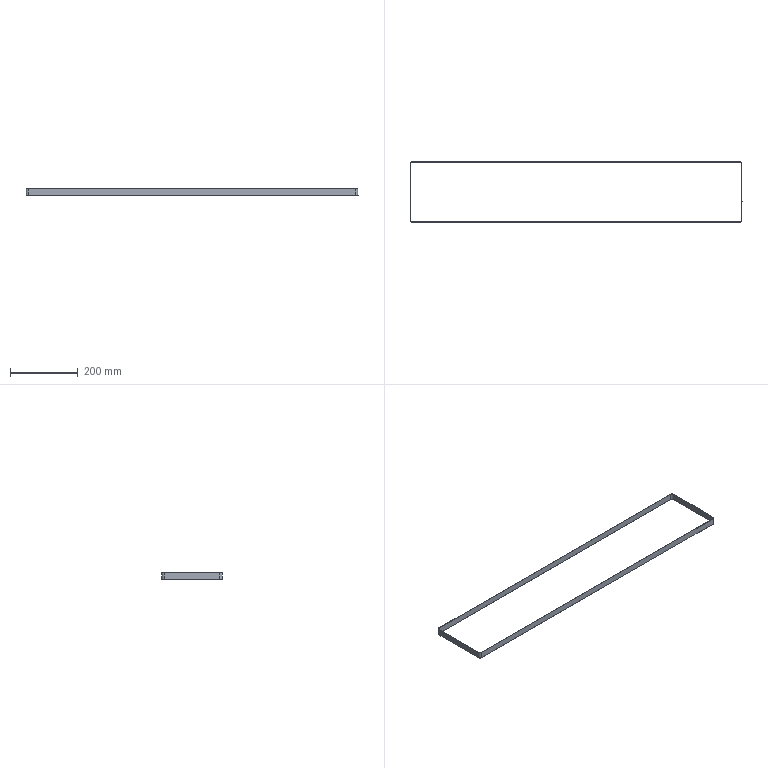Part | NX | features BREP 1 | 1 solid | 26 faces | box 980.9 x 177.8 x 19 mm | volume 35873 mm3 | plane 16 | cylinder 10 | commonest cylinder face diameters 11 x4 12.6 x4 1.64 x2
STEP:
#1=CARTESIAN_POINT('',(483.7,-88.1,0.));
#2=VERTEX_POINT('',#1);
#3=CARTESIAN_POINT('',(483.7,-88.1,-19.));
#4=VERTEX_POINT('',#3);
#5=CARTESIAN_POINT('',(483.7,-88.1,-19.));
#6=DIRECTION('',(0.,0.,-1.));
#7=VECTOR('',#6,1000.);
#8=LINE('',#5,#7);
#9=EDGE_CURVE('',#2,#4,#8,.T.);
#10=ORIENTED_EDGE('',*,*,#9,.T.);
#11=CARTESIAN_POINT('',(-483.7,-88.1,-19.));
#12=VERTEX_POINT('',#11);
#13=CARTESIAN_POINT('',(-483.7,-88.1,-19.));
#14=DIRECTION('',(-1.,0.,0.));
#15=VECTOR('',#14,1000.);
#16=LINE('',#13,#15);
#17=EDGE_CURVE('',#4,#12,#16,.T.);
#18=ORIENTED_EDGE('',*,*,#17,.T.);
#19=CARTESIAN_POINT('',(-483.7,-88.1,0.));
#20=VERTEX_POINT('',#19);
#21=CARTESIAN_POINT('',(-483.7,-88.1,-19.));
#22=DIRECTION('',(0.,0.,1.));
#23=VECTOR('',#22,1000.);
#24=LINE('',#21,#23);
#25=EDGE_CURVE('',#12,#20,#24,.T.);
#26=ORIENTED_EDGE('',*,*,#25,.T.);
#27=CARTESIAN_POINT('',(-483.7,-88.1,0.));
#28=DIRECTION('',(1.,0.,0.));
#29=VECTOR('',#28,1000.);
#30=LINE('',#27,#29);
#31=EDGE_CURVE('',#20,#2,#30,.T.);
#32=ORIENTED_EDGE('',*,*,#31,.T.);
#33=EDGE_LOOP('',(#10,#18,#26,#32));
#34=FACE_BOUND('',#33,.T.);
#35=CARTESIAN_POINT('',(-483.7,-88.1,-19.));
#36=DIRECTION('',(0.,1.,0.));
#37=DIRECTION('',(0.,0.,-1.));
#38=AXIS2_PLACEMENT_3D('',#35,#36,#37);
#39=PLANE('',#38);
#40=ADVANCED_FACE('',(#34),#39,.T.);
#41=CARTESIAN_POINT('',(490.001,-28.898,-19.));
#42=VERTEX_POINT('',#41);
#43=CARTESIAN_POINT('',(490.,-82.6,-19.));
#44=VERTEX_POINT('',#43);
#45=CARTESIAN_POINT('',(490.,-82.6,-19.));
#46=DIRECTION('',(0.,-1.,0.));
#47=VECTOR('',#46,1000.);
#48=LINE('',#45,#47);
#49=EDGE_CURVE('',#42,#44,#48,.T.);
#50=ORIENTED_EDGE('',*,*,#49,.T.);
#51=CARTESIAN_POINT('',(483.7,-88.9,-19.));
#52=VERTEX_POINT('',#51);
#53=CARTESIAN_POINT('',(483.7,-82.6,-19.));
#54=DIRECTION('',(0.,0.,-1.));
#55=DIRECTION('',(1.,0.,0.));
#56=AXIS2_PLACEMENT_3D('',#53,#54,#55);
#57=CIRCLE('',#56,6.3);
#58=EDGE_CURVE('',#44,#52,#57,.T.);
#59=ORIENTED_EDGE('',*,*,#58,.T.);
#60=CARTESIAN_POINT('',(-483.7,-88.9,-19.));
#61=VERTEX_POINT('',#60);
#62=CARTESIAN_POINT('',(489.2,-88.9,-19.));
#63=DIRECTION('',(-1.,0.,0.));
#64=VECTOR('',#63,1000.);
#65=LINE('',#62,#64);
#66=EDGE_CURVE('',#52,#61,#65,.T.);
#67=ORIENTED_EDGE('',*,*,#66,.T.);
#68=CARTESIAN_POINT('',(-490.,-82.6,-19.));
#69=VERTEX_POINT('',#68);
#70=CARTESIAN_POINT('',(-483.7,-82.6,-19.));
#71=DIRECTION('',(0.,0.,-1.));
#72=DIRECTION('',(1.,0.,0.));
#73=AXIS2_PLACEMENT_3D('',#70,#71,#72);
#74=CIRCLE('',#73,6.3);
#75=EDGE_CURVE('',#61,#69,#74,.T.);
#76=ORIENTED_EDGE('',*,*,#75,.T.);
#77=CARTESIAN_POINT('',(-490.,82.6,-19.));
#78=VERTEX_POINT('',#77);
#79=CARTESIAN_POINT('',(-490.,-82.6,-19.));
#80=DIRECTION('',(0.,1.,0.));
#81=VECTOR('',#80,1000.);
#82=LINE('',#79,#81);
#83=EDGE_CURVE('',#69,#78,#82,.T.);
#84=ORIENTED_EDGE('',*,*,#83,.T.);
#85=CARTESIAN_POINT('',(-483.7,88.9,-19.));
#86=VERTEX_POINT('',#85);
#87=CARTESIAN_POINT('',(-483.7,82.6,-19.));
#88=DIRECTION('',(0.,0.,-1.));
#89=DIRECTION('',(1.,0.,0.));
#90=AXIS2_PLACEMENT_3D('',#87,#88,#89);
#91=CIRCLE('',#90,6.3);
#92=EDGE_CURVE('',#78,#86,#91,.T.);
#93=ORIENTED_EDGE('',*,*,#92,.T.);
#94=CARTESIAN_POINT('',(483.7,88.9,-19.));
#95=VERTEX_POINT('',#94);
#96=CARTESIAN_POINT('',(489.2,88.9,-19.));
#97=DIRECTION('',(1.,0.,0.));
#98=VECTOR('',#97,1000.);
#99=LINE('',#96,#98);
#100=EDGE_CURVE('',#86,#95,#99,.T.);
#101=ORIENTED_EDGE('',*,*,#100,.T.);
#102=CARTESIAN_POINT('',(490.,82.6,-19.));
#103=VERTEX_POINT('',#102);
#104=CARTESIAN_POINT('',(483.7,82.6,-19.));
#105=DIRECTION('',(0.,0.,-1.));
#106=DIRECTION('',(1.,0.,0.));
#107=AXIS2_PLACEMENT_3D('',#104,#105,#106);
#108=CIRCLE('',#107,6.3);
#109=EDGE_CURVE('',#95,#103,#108,.T.);
#110=ORIENTED_EDGE('',*,*,#109,.T.);
#111=CARTESIAN_POINT('',(490.,-26.1,-19.));
#112=VERTEX_POINT('',#111);
#113=CARTESIAN_POINT('',(490.,-82.6,-19.));
#114=DIRECTION('',(0.,-1.,0.));
#115=VECTOR('',#114,1000.);
#116=LINE('',#113,#115);
#117=EDGE_CURVE('',#103,#112,#116,.T.);
#118=ORIENTED_EDGE('',*,*,#117,.T.);
#119=CARTESIAN_POINT('',(489.2,-26.1,-19.));
#120=VERTEX_POINT('',#119);
#121=CARTESIAN_POINT('',(490.,-26.1,-19.));
#122=DIRECTION('',(1.,0.,0.));
#123=VECTOR('',#122,1000.);
#124=LINE('',#121,#123);
#125=EDGE_CURVE('',#120,#112,#124,.T.);
#126=ORIENTED_EDGE('',*,*,#125,.F.);
#127=CARTESIAN_POINT('',(489.2,82.6,-19.));
#128=VERTEX_POINT('',#127);
#129=CARTESIAN_POINT('',(489.2,-82.6,-19.));
#130=DIRECTION('',(0.,1.,0.));
#131=VECTOR('',#130,1000.);
#132=LINE('',#129,#131);
#133=EDGE_CURVE('',#120,#128,#132,.T.);
#134=ORIENTED_EDGE('',*,*,#133,.T.);
#135=CARTESIAN_POINT('',(483.7,88.1,-19.));
#136=VERTEX_POINT('',#135);
#137=CARTESIAN_POINT('',(483.7,82.6,-19.));
#138=DIRECTION('',(0.,0.,1.));
#139=DIRECTION('',(1.,0.,0.));
#140=AXIS2_PLACEMENT_3D('',#137,#138,#139);
#141=CIRCLE('',#140,5.5);
#142=EDGE_CURVE('',#128,#136,#141,.T.);
#143=ORIENTED_EDGE('',*,*,#142,.T.);
#144=CARTESIAN_POINT('',(-483.7,88.1,-19.));
#145=VERTEX_POINT('',#144);
#146=CARTESIAN_POINT('',(489.2,88.1,-19.));
#147=DIRECTION('',(-1.,0.,0.));
#148=VECTOR('',#147,1000.);
#149=LINE('',#146,#148);
#150=EDGE_CURVE('',#136,#145,#149,.T.);
#151=ORIENTED_EDGE('',*,*,#150,.T.);
#152=CARTESIAN_POINT('',(-489.2,82.6,-19.));
#153=VERTEX_POINT('',#152);
#154=CARTESIAN_POINT('',(-483.7,82.6,-19.));
#155=DIRECTION('',(0.,0.,1.));
#156=DIRECTION('',(1.,0.,0.));
#157=AXIS2_PLACEMENT_3D('',#154,#155,#156);
#158=CIRCLE('',#157,5.5);
#159=EDGE_CURVE('',#145,#153,#158,.T.);
#160=ORIENTED_EDGE('',*,*,#159,.T.);
#161=CARTESIAN_POINT('',(-489.2,-82.6,-19.));
#162=VERTEX_POINT('',#161);
#163=CARTESIAN_POINT('',(-489.2,-82.6,-19.));
#164=DIRECTION('',(0.,-1.,0.));
#165=VECTOR('',#164,1000.);
#166=LINE('',#163,#165);
#167=EDGE_CURVE('',#153,#162,#166,.T.);
#168=ORIENTED_EDGE('',*,*,#167,.T.);
#169=CARTESIAN_POINT('',(-483.7,-82.6,-19.));
#170=DIRECTION('',(0.,0.,1.));
#171=DIRECTION('',(1.,0.,0.));
#172=AXIS2_PLACEMENT_3D('',#169,#170,#171);
#173=CIRCLE('',#172,5.5);
#174=EDGE_CURVE('',#162,#12,#173,.T.);
#175=ORIENTED_EDGE('',*,*,#174,.T.);
#176=ORIENTED_EDGE('',*,*,#17,.F.);
#177=CARTESIAN_POINT('',(489.2,-82.6,-19.));
#178=VERTEX_POINT('',#177);
#179=CARTESIAN_POINT('',(483.7,-82.6,-19.));
#180=DIRECTION('',(0.,0.,1.));
#181=DIRECTION('',(1.,0.,0.));
#182=AXIS2_PLACEMENT_3D('',#179,#180,#181);
#183=CIRCLE('',#182,5.5);
#184=EDGE_CURVE('',#4,#178,#183,.T.);
#185=ORIENTED_EDGE('',*,*,#184,.T.);
#186=CARTESIAN_POINT('',(489.2,-28.92,-19.));
#187=VERTEX_POINT('',#186);
#188=CARTESIAN_POINT('',(489.2,-82.6,-19.));
#189=DIRECTION('',(0.,1.,0.));
#190=VECTOR('',#189,1000.);
#191=LINE('',#188,#190);
#192=EDGE_CURVE('',#178,#187,#191,.T.);
#193=ORIENTED_EDGE('',*,*,#192,.T.);
#194=CARTESIAN_POINT('',(490.099,-28.104,-19.));
#195=VERTEX_POINT('',#194);
#196=CARTESIAN_POINT('',(490.02,-28.92,-19.));
#197=DIRECTION('',(0.,0.,1.));
#198=DIRECTION('',(1.,0.,0.));
#199=AXIS2_PLACEMENT_3D('',#196,#197,#198);
#200=CIRCLE('',#199,0.82);
#201=EDGE_CURVE('',#195,#187,#200,.T.);
#202=ORIENTED_EDGE('',*,*,#201,.F.);
#203=CARTESIAN_POINT('',(490.1,31.9,-19.));
#204=VERTEX_POINT('',#203);
#205=CARTESIAN_POINT('',(490.1,-82.6,-19.));
#206=DIRECTION('',(0.,1.,0.));
#207=VECTOR('',#206,1000.);
#208=LINE('',#205,#207);
#209=EDGE_CURVE('',#195,#204,#208,.T.);
#210=ORIENTED_EDGE('',*,*,#209,.T.);
#211=CARTESIAN_POINT('',(490.9,31.9,-19.));
#212=VERTEX_POINT('',#211);
#213=CARTESIAN_POINT('',(490.1,31.9,-19.));
#214=DIRECTION('',(-1.,0.,0.));
#215=VECTOR('',#214,1000.);
#216=LINE('',#213,#215);
#217=EDGE_CURVE('',#212,#204,#216,.T.);
#218=ORIENTED_EDGE('',*,*,#217,.F.);
#219=CARTESIAN_POINT('',(490.9,-28.08,-19.));
#220=VERTEX_POINT('',#219);
#221=CARTESIAN_POINT('',(490.9,-82.6,-19.));
#222=DIRECTION('',(0.,-1.,0.));
#223=VECTOR('',#222,1000.);
#224=LINE('',#221,#223);
#225=EDGE_CURVE('',#212,#220,#224,.T.);
#226=ORIENTED_EDGE('',*,*,#225,.T.);
#227=CARTESIAN_POINT('',(490.08,-28.08,-19.));
#228=DIRECTION('',(0.,0.,1.));
#229=DIRECTION('',(1.,0.,0.));
#230=AXIS2_PLACEMENT_3D('',#227,#228,#229);
#231=CIRCLE('',#230,0.82);
#232=EDGE_CURVE('',#42,#220,#231,.T.);
#233=ORIENTED_EDGE('',*,*,#232,.F.);
#234=EDGE_LOOP('',(#50,#59,#67,#76,#84,#93,#101,#110,#118,#126,#134,#143,#151,#160,#168,#175,#176,#185,#193,#202,#210,#218,#226,#233));
#235=FACE_BOUND('',#234,.T.);
#236=CARTESIAN_POINT('',(489.2,-82.6,-19.));
#237=DIRECTION('',(0.,0.,-1.));
#238=DIRECTION('',(1.,0.,0.));
#239=AXIS2_PLACEMENT_3D('',#236,#237,#238);
#240=PLANE('',#239);
#241=ADVANCED_FACE('',(#235),#240,.T.);
#242=ORIENTED_EDGE('',*,*,#9,.F.);
#243=CARTESIAN_POINT('',(489.2,-82.6,0.));
#244=VERTEX_POINT('',#243);
#245=CARTESIAN_POINT('',(483.7,-82.6,0.));
#246=DIRECTION('',(0.,0.,-1.));
#247=DIRECTION('',(1.,0.,0.));
#248=AXIS2_PLACEMENT_3D('',#245,#246,#247);
#249=CIRCLE('',#248,5.5);
#250=EDGE_CURVE('',#244,#2,#249,.T.);
#251=ORIENTED_EDGE('',*,*,#250,.F.);
#252=CARTESIAN_POINT('',(489.2,-82.6,-19.));
#253=DIRECTION('',(0.,0.,1.));
#254=VECTOR('',#253,1000.);
#255=LINE('',#252,#254);
#256=EDGE_CURVE('',#178,#244,#255,.T.);
#257=ORIENTED_EDGE('',*,*,#256,.F.);
#258=ORIENTED_EDGE('',*,*,#184,.F.);
#259=EDGE_LOOP('',(#242,#251,#257,#258));
#260=FACE_BOUND('',#259,.T.);
#261=CARTESIAN_POINT('',(483.7,-82.6,-19.));
#262=DIRECTION('',(0.,0.,1.));
#263=DIRECTION('',(-1.,0.,0.));
#264=AXIS2_PLACEMENT_3D('',#261,#262,#263);
#265=CYLINDRICAL_SURFACE('',#264,5.5);
#266=ADVANCED_FACE('',(#260),#265,.F.);
#267=CARTESIAN_POINT('',(-490.,82.6,0.));
#268=VERTEX_POINT('',#267);
#269=CARTESIAN_POINT('',(-490.,-82.6,0.));
#270=VERTEX_POINT('',#269);
#271=CARTESIAN_POINT('',(-490.,-88.1,0.));
#272=DIRECTION('',(0.,-1.,0.));
#273=VECTOR('',#272,1000.);
#274=LINE('',#271,#273);
#275=EDGE_CURVE('',#268,#270,#274,.T.);
#276=ORIENTED_EDGE('',*,*,#275,.T.);
#277=CARTESIAN_POINT('',(-483.7,-88.9,0.));
#278=VERTEX_POINT('',#277);
#279=CARTESIAN_POINT('',(-483.7,-82.6,0.));
#280=DIRECTION('',(0.,0.,1.));
#281=DIRECTION('',(1.,0.,0.));
#282=AXIS2_PLACEMENT_3D('',#279,#280,#281);
#283=CIRCLE('',#282,6.3);
#284=EDGE_CURVE('',#270,#278,#283,.T.);
#285=ORIENTED_EDGE('',*,*,#284,.T.);
#286=CARTESIAN_POINT('',(483.7,-88.9,0.));
#287=VERTEX_POINT('',#286);
#288=CARTESIAN_POINT('',(483.7,-88.9,0.));
#289=DIRECTION('',(1.,0.,0.));
#290=VECTOR('',#289,1000.);
#291=LINE('',#288,#290);
#292=EDGE_CURVE('',#278,#287,#291,.T.);
#293=ORIENTED_EDGE('',*,*,#292,.T.);
#294=CARTESIAN_POINT('',(490.,-82.6,0.));
#295=VERTEX_POINT('',#294);
#296=CARTESIAN_POINT('',(483.7,-82.6,0.));
#297=DIRECTION('',(0.,0.,1.));
#298=DIRECTION('',(1.,0.,0.));
#299=AXIS2_PLACEMENT_3D('',#296,#297,#298);
#300=CIRCLE('',#299,6.3);
#301=EDGE_CURVE('',#287,#295,#300,.T.);
#302=ORIENTED_EDGE('',*,*,#301,.T.);
#303=CARTESIAN_POINT('',(490.001,-28.898,0.));
#304=VERTEX_POINT('',#303);
#305=CARTESIAN_POINT('',(490.,-82.6,0.));
#306=DIRECTION('',(0.,1.,0.));
#307=VECTOR('',#306,1000.);
#308=LINE('',#305,#307);
#309=EDGE_CURVE('',#295,#304,#308,.T.);
#310=ORIENTED_EDGE('',*,*,#309,.T.);
#311=CARTESIAN_POINT('',(490.9,-28.08,0.));
#312=VERTEX_POINT('',#311);
#313=CARTESIAN_POINT('',(490.08,-28.08,0.));
#314=DIRECTION('',(0.,0.,-1.));
#315=DIRECTION('',(1.,0.,0.));
#316=AXIS2_PLACEMENT_3D('',#313,#314,#315);
#317=CIRCLE('',#316,0.82);
#318=EDGE_CURVE('',#312,#304,#317,.T.);
#319=ORIENTED_EDGE('',*,*,#318,.F.);
#320=CARTESIAN_POINT('',(490.9,31.9,0.));
#321=VERTEX_POINT('',#320);
#322=CARTESIAN_POINT('',(490.9,-88.1,0.));
#323=DIRECTION('',(0.,1.,0.));
#324=VECTOR('',#323,1000.);
#325=LINE('',#322,#324);
#326=EDGE_CURVE('',#312,#321,#325,.T.);
#327=ORIENTED_EDGE('',*,*,#326,.T.);
#328=CARTESIAN_POINT('',(490.1,31.9,0.));
#329=VERTEX_POINT('',#328);
#330=CARTESIAN_POINT('',(490.1,31.9,0.));
#331=DIRECTION('',(1.,0.,0.));
#332=VECTOR('',#331,1000.);
#333=LINE('',#330,#332);
#334=EDGE_CURVE('',#329,#321,#333,.T.);
#335=ORIENTED_EDGE('',*,*,#334,.F.);
#336=CARTESIAN_POINT('',(490.099,-28.104,0.));
#337=VERTEX_POINT('',#336);
#338=CARTESIAN_POINT('',(490.1,-88.1,0.));
#339=DIRECTION('',(0.,-1.,0.));
#340=VECTOR('',#339,1000.);
#341=LINE('',#338,#340);
#342=EDGE_CURVE('',#329,#337,#341,.T.);
#343=ORIENTED_EDGE('',*,*,#342,.T.);
#344=CARTESIAN_POINT('',(489.2,-28.92,0.));
#345=VERTEX_POINT('',#344);
#346=CARTESIAN_POINT('',(490.02,-28.92,0.));
#347=DIRECTION('',(0.,0.,-1.));
#348=DIRECTION('',(1.,0.,0.));
#349=AXIS2_PLACEMENT_3D('',#346,#347,#348);
#350=CIRCLE('',#349,0.82);
#351=EDGE_CURVE('',#345,#337,#350,.T.);
#352=ORIENTED_EDGE('',*,*,#351,.F.);
#353=CARTESIAN_POINT('',(489.2,-88.1,0.));
#354=DIRECTION('',(0.,-1.,0.));
#355=VECTOR('',#354,1000.);
#356=LINE('',#353,#355);
#357=EDGE_CURVE('',#345,#244,#356,.T.);
#358=ORIENTED_EDGE('',*,*,#357,.T.);
#359=ORIENTED_EDGE('',*,*,#250,.T.);
#360=ORIENTED_EDGE('',*,*,#31,.F.);
#361=CARTESIAN_POINT('',(-489.2,-82.6,0.));
#362=VERTEX_POINT('',#361);
#363=CARTESIAN_POINT('',(-483.7,-82.6,0.));
#364=DIRECTION('',(0.,0.,-1.));
#365=DIRECTION('',(1.,0.,0.));
#366=AXIS2_PLACEMENT_3D('',#363,#364,#365);
#367=CIRCLE('',#366,5.5);
#368=EDGE_CURVE('',#20,#362,#367,.T.);
#369=ORIENTED_EDGE('',*,*,#368,.T.);
#370=CARTESIAN_POINT('',(-489.2,82.6,0.));
#371=VERTEX_POINT('',#370);
#372=CARTESIAN_POINT('',(-489.2,-88.1,0.));
#373=DIRECTION('',(0.,1.,0.));
#374=VECTOR('',#373,1000.);
#375=LINE('',#372,#374);
#376=EDGE_CURVE('',#362,#371,#375,.T.);
#377=ORIENTED_EDGE('',*,*,#376,.T.);
#378=CARTESIAN_POINT('',(-483.7,88.1,0.));
#379=VERTEX_POINT('',#378);
#380=CARTESIAN_POINT('',(-483.7,82.6,0.));
#381=DIRECTION('',(0.,0.,-1.));
#382=DIRECTION('',(1.,0.,0.));
#383=AXIS2_PLACEMENT_3D('',#380,#381,#382);
#384=CIRCLE('',#383,5.5);
#385=EDGE_CURVE('',#371,#379,#384,.T.);
#386=ORIENTED_EDGE('',*,*,#385,.T.);
#387=CARTESIAN_POINT('',(483.7,88.1,0.));
#388=VERTEX_POINT('',#387);
#389=CARTESIAN_POINT('',(483.7,88.1,0.));
#390=DIRECTION('',(1.,0.,0.));
#391=VECTOR('',#390,1000.);
#392=LINE('',#389,#391);
#393=EDGE_CURVE('',#379,#388,#392,.T.);
#394=ORIENTED_EDGE('',*,*,#393,.T.);
#395=CARTESIAN_POINT('',(489.2,82.6,0.));
#396=VERTEX_POINT('',#395);
#397=CARTESIAN_POINT('',(483.7,82.6,0.));
#398=DIRECTION('',(0.,0.,-1.));
#399=DIRECTION('',(1.,0.,0.));
#400=AXIS2_PLACEMENT_3D('',#397,#398,#399);
#401=CIRCLE('',#400,5.5);
#402=EDGE_CURVE('',#388,#396,#401,.T.);
#403=ORIENTED_EDGE('',*,*,#402,.T.);
#404=CARTESIAN_POINT('',(489.2,-26.1,0.));
#405=VERTEX_POINT('',#404);
#406=CARTESIAN_POINT('',(489.2,-88.1,0.));
#407=DIRECTION('',(0.,-1.,0.));
#408=VECTOR('',#407,1000.);
#409=LINE('',#406,#408);
#410=EDGE_CURVE('',#396,#405,#409,.T.);
#411=ORIENTED_EDGE('',*,*,#410,.T.);
#412=CARTESIAN_POINT('',(490.,-26.1,0.));
#413=VERTEX_POINT('',#412);
#414=CARTESIAN_POINT('',(490.,-26.1,0.));
#415=DIRECTION('',(-1.,0.,0.));
#416=VECTOR('',#415,1000.);
#417=LINE('',#414,#416);
#418=EDGE_CURVE('',#413,#405,#417,.T.);
#419=ORIENTED_EDGE('',*,*,#418,.F.);
#420=CARTESIAN_POINT('',(490.,82.6,0.));
#421=VERTEX_POINT('',#420);
#422=CARTESIAN_POINT('',(490.,-88.1,0.));
#423=DIRECTION('',(0.,1.,0.));
#424=VECTOR('',#423,1000.);
#425=LINE('',#422,#424);
#426=EDGE_CURVE('',#413,#421,#425,.T.);
#427=ORIENTED_EDGE('',*,*,#426,.T.);
#428=CARTESIAN_POINT('',(483.7,88.9,0.));
#429=VERTEX_POINT('',#428);
#430=CARTESIAN_POINT('',(483.7,82.6,0.));
#431=DIRECTION('',(0.,0.,1.));
#432=DIRECTION('',(1.,0.,0.));
#433=AXIS2_PLACEMENT_3D('',#430,#431,#432);
#434=CIRCLE('',#433,6.3);
#435=EDGE_CURVE('',#421,#429,#434,.T.);
#436=ORIENTED_EDGE('',*,*,#435,.T.);
#437=CARTESIAN_POINT('',(-483.7,88.9,0.));
#438=VERTEX_POINT('',#437);
#439=CARTESIAN_POINT('',(483.7,88.9,0.));
#440=DIRECTION('',(-1.,0.,0.));
#441=VECTOR('',#440,1000.);
#442=LINE('',#439,#441);
#443=EDGE_CURVE('',#429,#438,#442,.T.);
#444=ORIENTED_EDGE('',*,*,#443,.T.);
#445=CARTESIAN_POINT('',(-483.7,82.6,0.));
#446=DIRECTION('',(0.,0.,1.));
#447=DIRECTION('',(1.,0.,0.));
#448=AXIS2_PLACEMENT_3D('',#445,#446,#447);
#449=CIRCLE('',#448,6.3);
#450=EDGE_CURVE('',#438,#268,#449,.T.);
#451=ORIENTED_EDGE('',*,*,#450,.T.);
#452=EDGE_LOOP('',(#276,#285,#293,#302,#310,#319,#327,#335,#343,#352,#358,#359,#360,#369,#377,#386,#394,#403,#411,#419,#427,#436,#444,#451));
#453=FACE_BOUND('',#452,.T.);
#454=CARTESIAN_POINT('',(483.7,-88.1,0.));
#455=DIRECTION('',(0.,0.,1.));
#456=DIRECTION('',(-1.,0.,0.));
#457=AXIS2_PLACEMENT_3D('',#454,#455,#456);
#458=PLANE('',#457);
#459=ADVANCED_FACE('',(#453),#458,.T.);
#460=CARTESIAN_POINT('',(-489.2,-82.6,-19.));
#461=DIRECTION('',(0.,0.,-1.));
#462=VECTOR('',#461,1000.);
#463=LINE('',#460,#462);
#464=EDGE_CURVE('',#362,#162,#463,.T.);
#465=ORIENTED_EDGE('',*,*,#464,.F.);
#466=ORIENTED_EDGE('',*,*,#368,.F.);
#467=ORIENTED_EDGE('',*,*,#25,.F.);
#468=ORIENTED_EDGE('',*,*,#174,.F.);
#469=EDGE_LOOP('',(#465,#466,#467,#468));
#470=FACE_BOUND('',#469,.T.);
#471=CARTESIAN_POINT('',(-483.7,-82.6,-19.));
#472=DIRECTION('',(0.,0.,1.));
#473=DIRECTION('',(-1.,0.,0.));
#474=AXIS2_PLACEMENT_3D('',#471,#472,#473);
#475=CYLINDRICAL_SURFACE('',#474,5.5);
#476=ADVANCED_FACE('',(#470),#475,.F.);
#477=CARTESIAN_POINT('',(483.7,-88.9,-19.));
#478=DIRECTION('',(0.,0.,-1.));
#479=VECTOR('',#478,1000.);
#480=LINE('',#477,#479);
#481=EDGE_CURVE('',#287,#52,#480,.T.);
#482=ORIENTED_EDGE('',*,*,#481,.T.);
#483=ORIENTED_EDGE('',*,*,#58,.F.);
#484=CARTESIAN_POINT('',(490.,-82.6,-19.));
#485=DIRECTION('',(0.,0.,1.));
#486=VECTOR('',#485,1000.);
#487=LINE('',#484,#486);
#488=EDGE_CURVE('',#44,#295,#487,.T.);
#489=ORIENTED_EDGE('',*,*,#488,.T.);
#490=ORIENTED_EDGE('',*,*,#301,.F.);
#491=EDGE_LOOP('',(#482,#483,#489,#490));
#492=FACE_BOUND('',#491,.T.);
#493=CARTESIAN_POINT('',(483.7,-82.6,-19.));
#494=DIRECTION('',(0.,0.,1.));
#495=DIRECTION('',(-1.,0.,0.));
#496=AXIS2_PLACEMENT_3D('',#493,#494,#495);
#497=CYLINDRICAL_SURFACE('',#496,6.3);
#498=ADVANCED_FACE('',(#492),#497,.T.);
#499=CARTESIAN_POINT('',(490.,-28.896,0.));
#500=DIRECTION('',(0.,0.,-1.));
#501=VECTOR('',#500,1000.);
#502=LINE('',#499,#501);
#503=EDGE_CURVE('',#304,#42,#502,.T.);
#504=ORIENTED_EDGE('',*,*,#503,.F.);
#505=ORIENTED_EDGE('',*,*,#309,.F.);
#506=ORIENTED_EDGE('',*,*,#488,.F.);
#507=ORIENTED_EDGE('',*,*,#49,.F.);
#508=EDGE_LOOP('',(#504,#505,#506,#507));
#509=FACE_BOUND('',#508,.T.);
#510=CARTESIAN_POINT('',(490.,-82.6,-19.));
#511=DIRECTION('',(-1.,0.,0.));
#512=DIRECTION('',(0.,0.,-1.));
#513=AXIS2_PLACEMENT_3D('',#510,#511,#512);
#514=PLANE('',#513);
#515=ADVANCED_FACE('',(#509),#514,.F.);
#516=CARTESIAN_POINT('',(490.9,31.9,-19.));
#517=DIRECTION('',(0.,0.,-1.));
#518=VECTOR('',#517,1000.);
#519=LINE('',#516,#518);
#520=EDGE_CURVE('',#321,#212,#519,.T.);
#521=ORIENTED_EDGE('',*,*,#520,.F.);
#522=ORIENTED_EDGE('',*,*,#326,.F.);
#523=CARTESIAN_POINT('',(490.9,-28.08,-19.));
#524=DIRECTION('',(0.,0.,1.));
#525=VECTOR('',#524,1000.);
#526=LINE('',#523,#525);
#527=EDGE_CURVE('',#220,#312,#526,.T.);
#528=ORIENTED_EDGE('',*,*,#527,.F.);
#529=ORIENTED_EDGE('',*,*,#225,.F.);
#530=EDGE_LOOP('',(#521,#522,#528,#529));
#531=FACE_BOUND('',#530,.T.);
#532=CARTESIAN_POINT('',(490.9,-28.1,-19.));
#533=DIRECTION('',(-1.,0.,0.));
#534=DIRECTION('',(0.,0.,-1.));
#535=AXIS2_PLACEMENT_3D('',#532,#533,#534);
#536=PLANE('',#535);
#537=ADVANCED_FACE('',(#531),#536,.F.);
#538=CARTESIAN_POINT('',(490.1,31.9,-19.));
#539=DIRECTION('',(0.,0.,-1.));
#540=VECTOR('',#539,1000.);
#541=LINE('',#538,#540);
#542=EDGE_CURVE('',#329,#204,#541,.T.);
#543=ORIENTED_EDGE('',*,*,#542,.T.);
#544=ORIENTED_EDGE('',*,*,#209,.F.);
#545=CARTESIAN_POINT('',(490.1,-28.104,-19.));
#546=DIRECTION('',(0.,0.,1.));
#547=VECTOR('',#546,1000.);
#548=LINE('',#545,#547);
#549=EDGE_CURVE('',#195,#337,#548,.T.);
#550=ORIENTED_EDGE('',*,*,#549,.T.);
#551=ORIENTED_EDGE('',*,*,#342,.F.);
#552=EDGE_LOOP('',(#543,#544,#550,#551));
#553=FACE_BOUND('',#552,.T.);
#554=CARTESIAN_POINT('',(490.1,-28.1,-19.));
#555=DIRECTION('',(-1.,0.,0.));
#556=DIRECTION('',(0.,0.,-1.));
#557=AXIS2_PLACEMENT_3D('',#554,#555,#556);
#558=PLANE('',#557);
#559=ADVANCED_FACE('',(#553),#558,.T.);
#560=CARTESIAN_POINT('',(489.2,-28.92,-19.));
#561=DIRECTION('',(0.,0.,-1.));
#562=VECTOR('',#561,1000.);
#563=LINE('',#560,#562);
#564=EDGE_CURVE('',#345,#187,#563,.T.);
#565=ORIENTED_EDGE('',*,*,#564,.T.);
#566=ORIENTED_EDGE('',*,*,#192,.F.);
#567=ORIENTED_EDGE('',*,*,#256,.T.);
#568=ORIENTED_EDGE('',*,*,#357,.F.);
#569=EDGE_LOOP('',(#565,#566,#567,#568));
#570=FACE_BOUND('',#569,.T.);
#571=CARTESIAN_POINT('',(489.2,-82.6,-19.));
#572=DIRECTION('',(-1.,0.,0.));
#573=DIRECTION('',(0.,0.,-1.));
#574=AXIS2_PLACEMENT_3D('',#571,#572,#573);
#575=PLANE('',#574);
#576=ADVANCED_FACE('',(#570),#575,.T.);
#577=ORIENTED_EDGE('',*,*,#464,.T.);
#578=ORIENTED_EDGE('',*,*,#167,.F.);
#579=CARTESIAN_POINT('',(-489.2,82.6,-19.));
#580=DIRECTION('',(0.,0.,1.));
#581=VECTOR('',#580,1000.);
#582=LINE('',#579,#581);
#583=EDGE_CURVE('',#153,#371,#582,.T.);
#584=ORIENTED_EDGE('',*,*,#583,.T.);
#585=ORIENTED_EDGE('',*,*,#376,.F.);
#586=EDGE_LOOP('',(#577,#578,#584,#585));
#587=FACE_BOUND('',#586,.T.);
#588=CARTESIAN_POINT('',(-489.2,-82.6,-19.));
#589=DIRECTION('',(1.,0.,0.));
#590=DIRECTION('',(0.,0.,1.));
#591=AXIS2_PLACEMENT_3D('',#588,#589,#590);
#592=PLANE('',#591);
#593=ADVANCED_FACE('',(#587),#592,.T.);
#594=CARTESIAN_POINT('',(-483.7,88.1,-19.));
#595=DIRECTION('',(0.,0.,-1.));
#596=VECTOR('',#595,1000.);
#597=LINE('',#594,#596);
#598=EDGE_CURVE('',#379,#145,#597,.T.);
#599=ORIENTED_EDGE('',*,*,#598,.F.);
#600=ORIENTED_EDGE('',*,*,#385,.F.);
#601=ORIENTED_EDGE('',*,*,#583,.F.);
#602=ORIENTED_EDGE('',*,*,#159,.F.);
#603=EDGE_LOOP('',(#599,#600,#601,#602));
#604=FACE_BOUND('',#603,.T.);
#605=CARTESIAN_POINT('',(-483.7,82.6,-19.));
#606=DIRECTION('',(0.,0.,1.));
#607=DIRECTION('',(-1.,0.,0.));
#608=AXIS2_PLACEMENT_3D('',#605,#606,#607);
#609=CYLINDRICAL_SURFACE('',#608,5.5);
#610=ADVANCED_FACE('',(#604),#609,.F.);
#611=ORIENTED_EDGE('',*,*,#598,.T.);
#612=ORIENTED_EDGE('',*,*,#150,.F.);
#613=CARTESIAN_POINT('',(483.7,88.1,-19.));
#614=DIRECTION('',(0.,0.,1.));
#615=VECTOR('',#614,1000.);
#616=LINE('',#613,#615);
#617=EDGE_CURVE('',#136,#388,#616,.T.);
#618=ORIENTED_EDGE('',*,*,#617,.T.);
#619=ORIENTED_EDGE('',*,*,#393,.F.);
#620=EDGE_LOOP('',(#611,#612,#618,#619));
#621=FACE_BOUND('',#620,.T.);
#622=CARTESIAN_POINT('',(-483.7,88.1,-19.));
#623=DIRECTION('',(0.,-1.,0.));
#624=DIRECTION('',(0.,0.,1.));
#625=AXIS2_PLACEMENT_3D('',#622,#623,#624);
#626=PLANE('',#625);
#627=ADVANCED_FACE('',(#621),#626,.T.);
#628=CARTESIAN_POINT('',(489.2,82.6,-19.));
#629=DIRECTION('',(0.,0.,-1.));
#630=VECTOR('',#629,1000.);
#631=LINE('',#628,#630);
#632=EDGE_CURVE('',#396,#128,#631,.T.);
#633=ORIENTED_EDGE('',*,*,#632,.F.);
#634=ORIENTED_EDGE('',*,*,#402,.F.);
#635=ORIENTED_EDGE('',*,*,#617,.F.);
#636=ORIENTED_EDGE('',*,*,#142,.F.);
#637=EDGE_LOOP('',(#633,#634,#635,#636));
#638=FACE_BOUND('',#637,.T.);
#639=CARTESIAN_POINT('',(483.7,82.6,-19.));
#640=DIRECTION('',(0.,0.,1.));
#641=DIRECTION('',(-1.,0.,0.));
#642=AXIS2_PLACEMENT_3D('',#639,#640,#641);
#643=CYLINDRICAL_SURFACE('',#642,5.5);
#644=ADVANCED_FACE('',(#638),#643,.F.);
#645=ORIENTED_EDGE('',*,*,#632,.T.);
#646=ORIENTED_EDGE('',*,*,#133,.F.);
#647=CARTESIAN_POINT('',(489.2,-26.1,-19.));
#648=DIRECTION('',(0.,0.,1.));
#649=VECTOR('',#648,1000.);
#650=LINE('',#647,#649);
#651=EDGE_CURVE('',#120,#405,#650,.T.);
#652=ORIENTED_EDGE('',*,*,#651,.T.);
#653=ORIENTED_EDGE('',*,*,#410,.F.);
#654=EDGE_LOOP('',(#645,#646,#652,#653));
#655=FACE_BOUND('',#654,.T.);
#656=CARTESIAN_POINT('',(489.2,-82.6,-19.));
#657=DIRECTION('',(-1.,0.,0.));
#658=DIRECTION('',(0.,0.,-1.));
#659=AXIS2_PLACEMENT_3D('',#656,#657,#658);
#660=PLANE('',#659);
#661=ADVANCED_FACE('',(#655),#660,.T.);
#662=CARTESIAN_POINT('',(490.,82.6,-19.));
#663=DIRECTION('',(0.,0.,-1.));
#664=VECTOR('',#663,1000.);
#665=LINE('',#662,#664);
#666=EDGE_CURVE('',#421,#103,#665,.T.);
#667=ORIENTED_EDGE('',*,*,#666,.F.);
#668=ORIENTED_EDGE('',*,*,#426,.F.);
#669=CARTESIAN_POINT('',(490.,-26.1,-19.));
#670=DIRECTION('',(0.,0.,1.));
#671=VECTOR('',#670,1000.);
#672=LINE('',#669,#671);
#673=EDGE_CURVE('',#112,#413,#672,.T.);
#674=ORIENTED_EDGE('',*,*,#673,.F.);
#675=ORIENTED_EDGE('',*,*,#117,.F.);
#676=EDGE_LOOP('',(#667,#668,#674,#675));
#677=FACE_BOUND('',#676,.T.);
#678=CARTESIAN_POINT('',(490.,-82.6,-19.));
#679=DIRECTION('',(-1.,0.,0.));
#680=DIRECTION('',(0.,0.,-1.));
#681=AXIS2_PLACEMENT_3D('',#678,#679,#680);
#682=PLANE('',#681);
#683=ADVANCED_FACE('',(#677),#682,.F.);
#684=ORIENTED_EDGE('',*,*,#666,.T.);
#685=ORIENTED_EDGE('',*,*,#109,.F.);
#686=CARTESIAN_POINT('',(483.7,88.9,-19.));
#687=DIRECTION('',(0.,0.,1.));
#688=VECTOR('',#687,1000.);
#689=LINE('',#686,#688);
#690=EDGE_CURVE('',#95,#429,#689,.T.);
#691=ORIENTED_EDGE('',*,*,#690,.T.);
#692=ORIENTED_EDGE('',*,*,#435,.F.);
#693=EDGE_LOOP('',(#684,#685,#691,#692));
#694=FACE_BOUND('',#693,.T.);
#695=CARTESIAN_POINT('',(483.7,82.6,-19.));
#696=DIRECTION('',(0.,0.,1.));
#697=DIRECTION('',(-1.,0.,0.));
#698=AXIS2_PLACEMENT_3D('',#695,#696,#697);
#699=CYLINDRICAL_SURFACE('',#698,6.3);
#700=ADVANCED_FACE('',(#694),#699,.T.);
#701=CARTESIAN_POINT('',(-483.7,88.9,-19.));
#702=DIRECTION('',(0.,0.,-1.));
#703=VECTOR('',#702,1000.);
#704=LINE('',#701,#703);
#705=EDGE_CURVE('',#438,#86,#704,.T.);
#706=ORIENTED_EDGE('',*,*,#705,.F.);
#707=ORIENTED_EDGE('',*,*,#443,.F.);
#708=ORIENTED_EDGE('',*,*,#690,.F.);
#709=ORIENTED_EDGE('',*,*,#100,.F.);
#710=EDGE_LOOP('',(#706,#707,#708,#709));
#711=FACE_BOUND('',#710,.T.);
#712=CARTESIAN_POINT('',(-483.7,88.9,-19.));
#713=DIRECTION('',(0.,-1.,0.));
#714=DIRECTION('',(0.,0.,1.));
#715=AXIS2_PLACEMENT_3D('',#712,#713,#714);
#716=PLANE('',#715);
#717=ADVANCED_FACE('',(#711),#716,.F.);
#718=ORIENTED_EDGE('',*,*,#705,.T.);
#719=ORIENTED_EDGE('',*,*,#92,.F.);
#720=CARTESIAN_POINT('',(-490.,82.6,-19.));
#721=DIRECTION('',(0.,0.,1.));
#722=VECTOR('',#721,1000.);
#723=LINE('',#720,#722);
#724=EDGE_CURVE('',#78,#268,#723,.T.);
#725=ORIENTED_EDGE('',*,*,#724,.T.);
#726=ORIENTED_EDGE('',*,*,#450,.F.);
#727=EDGE_LOOP('',(#718,#719,#725,#726));
#728=FACE_BOUND('',#727,.T.);
#729=CARTESIAN_POINT('',(-483.7,82.6,-19.));
#730=DIRECTION('',(0.,0.,1.));
#731=DIRECTION('',(-1.,0.,0.));
#732=AXIS2_PLACEMENT_3D('',#729,#730,#731);
#733=CYLINDRICAL_SURFACE('',#732,6.3);
#734=ADVANCED_FACE('',(#728),#733,.T.);
#735=CARTESIAN_POINT('',(-490.,-82.6,-19.));
#736=DIRECTION('',(0.,0.,-1.));
#737=VECTOR('',#736,1000.);
#738=LINE('',#735,#737);
#739=EDGE_CURVE('',#270,#69,#738,.T.);
#740=ORIENTED_EDGE('',*,*,#739,.F.);
#741=ORIENTED_EDGE('',*,*,#275,.F.);
#742=ORIENTED_EDGE('',*,*,#724,.F.);
#743=ORIENTED_EDGE('',*,*,#83,.F.);
#744=EDGE_LOOP('',(#740,#741,#742,#743));
#745=FACE_BOUND('',#744,.T.);
#746=CARTESIAN_POINT('',(-490.,-82.6,-19.));
#747=DIRECTION('',(1.,0.,0.));
#748=DIRECTION('',(0.,0.,1.));
#749=AXIS2_PLACEMENT_3D('',#746,#747,#748);
#750=PLANE('',#749);
#751=ADVANCED_FACE('',(#745),#750,.F.);
#752=ORIENTED_EDGE('',*,*,#739,.T.);
#753=ORIENTED_EDGE('',*,*,#75,.F.);
#754=CARTESIAN_POINT('',(-483.7,-88.9,-19.));
#755=DIRECTION('',(0.,0.,1.));
#756=VECTOR('',#755,1000.);
#757=LINE('',#754,#756);
#758=EDGE_CURVE('',#61,#278,#757,.T.);
#759=ORIENTED_EDGE('',*,*,#758,.T.);
#760=ORIENTED_EDGE('',*,*,#284,.F.);
#761=EDGE_LOOP('',(#752,#753,#759,#760));
#762=FACE_BOUND('',#761,.T.);
#763=CARTESIAN_POINT('',(-483.7,-82.6,-19.));
#764=DIRECTION('',(0.,0.,1.));
#765=DIRECTION('',(-1.,0.,0.));
#766=AXIS2_PLACEMENT_3D('',#763,#764,#765);
#767=CYLINDRICAL_SURFACE('',#766,6.3);
#768=ADVANCED_FACE('',(#762),#767,.T.);
#769=ORIENTED_EDGE('',*,*,#481,.F.);
#770=ORIENTED_EDGE('',*,*,#292,.F.);
#771=ORIENTED_EDGE('',*,*,#758,.F.);
#772=ORIENTED_EDGE('',*,*,#66,.F.);
#773=EDGE_LOOP('',(#769,#770,#771,#772));
#774=FACE_BOUND('',#773,.T.);
#775=CARTESIAN_POINT('',(-483.7,-88.9,-19.));
#776=DIRECTION('',(0.,1.,0.));
#777=DIRECTION('',(0.,0.,-1.));
#778=AXIS2_PLACEMENT_3D('',#775,#776,#777);
#779=PLANE('',#778);
#780=ADVANCED_FACE('',(#774),#779,.F.);
#781=ORIENTED_EDGE('',*,*,#503,.T.);
#782=ORIENTED_EDGE('',*,*,#232,.T.);
#783=ORIENTED_EDGE('',*,*,#527,.T.);
#784=ORIENTED_EDGE('',*,*,#318,.T.);
#785=EDGE_LOOP('',(#781,#782,#783,#784));
#786=FACE_BOUND('',#785,.T.);
#787=CARTESIAN_POINT('',(490.08,-28.08,-19.));
#788=DIRECTION('',(0.,0.,1.));
#789=DIRECTION('',(-1.,0.,0.));
#790=AXIS2_PLACEMENT_3D('',#787,#788,#789);
#791=CYLINDRICAL_SURFACE('',#790,0.82);
#792=ADVANCED_FACE('',(#786),#791,.T.);
#793=ORIENTED_EDGE('',*,*,#520,.T.);
#794=ORIENTED_EDGE('',*,*,#217,.T.);
#795=ORIENTED_EDGE('',*,*,#542,.F.);
#796=ORIENTED_EDGE('',*,*,#334,.T.);
#797=EDGE_LOOP('',(#793,#794,#795,#796));
#798=FACE_BOUND('',#797,.T.);
#799=CARTESIAN_POINT('',(490.1,31.9,-19.));
#800=DIRECTION('',(0.,1.,0.));
#801=DIRECTION('',(0.,0.,-1.));
#802=AXIS2_PLACEMENT_3D('',#799,#800,#801);
#803=PLANE('',#802);
#804=ADVANCED_FACE('',(#798),#803,.T.);
#805=ORIENTED_EDGE('',*,*,#549,.F.);
#806=ORIENTED_EDGE('',*,*,#201,.T.);
#807=ORIENTED_EDGE('',*,*,#564,.F.);
#808=ORIENTED_EDGE('',*,*,#351,.T.);
#809=EDGE_LOOP('',(#805,#806,#807,#808));
#810=FACE_BOUND('',#809,.T.);
#811=CARTESIAN_POINT('',(490.02,-28.92,-19.));
#812=DIRECTION('',(0.,0.,1.));
#813=DIRECTION('',(-1.,0.,0.));
#814=AXIS2_PLACEMENT_3D('',#811,#812,#813);
#815=CYLINDRICAL_SURFACE('',#814,0.82);
#816=ADVANCED_FACE('',(#810),#815,.T.);
#817=ORIENTED_EDGE('',*,*,#651,.F.);
#818=ORIENTED_EDGE('',*,*,#125,.T.);
#819=ORIENTED_EDGE('',*,*,#673,.T.);
#820=ORIENTED_EDGE('',*,*,#418,.T.);
#821=EDGE_LOOP('',(#817,#818,#819,#820));
#822=FACE_BOUND('',#821,.T.);
#823=CARTESIAN_POINT('',(490.,-26.1,-19.));
#824=DIRECTION('',(0.,-1.,0.));
#825=DIRECTION('',(0.,0.,1.));
#826=AXIS2_PLACEMENT_3D('',#823,#824,#825);
#827=PLANE('',#826);
#828=ADVANCED_FACE('',(#822),#827,.T.);
#829=CLOSED_SHELL('',(#40,#241,#266,#459,#476,#498,#515,#537,#559,#576,#593,#610,#627,#644,#661,#683,#700,#717,#734,#751,#768,#780,#792,#804,#816,#828));
#830=MANIFOLD_SOLID_BREP('',#829);
#831=(LENGTH_UNIT()NAMED_UNIT(*)SI_UNIT(.MILLI.,.METRE.));
#832=UNCERTAINTY_MEASURE_WITH_UNIT(LENGTH_MEASURE(0.00001),#831,'','');
#833=(NAMED_UNIT(*)PLANE_ANGLE_UNIT()SI_UNIT($,.RADIAN.));
#834=(NAMED_UNIT(*)SI_UNIT($,.STERADIAN.)SOLID_ANGLE_UNIT());
#835=(GEOMETRIC_REPRESENTATION_CONTEXT(3)GLOBAL_UNCERTAINTY_ASSIGNED_CONTEXT((#832))GLOBAL_UNIT_ASSIGNED_CONTEXT((#831,#833,#834))REPRESENTATION_CONTEXT('',''));
#836=ADVANCED_BREP_SHAPE_REPRESENTATION('',(#830),#835);